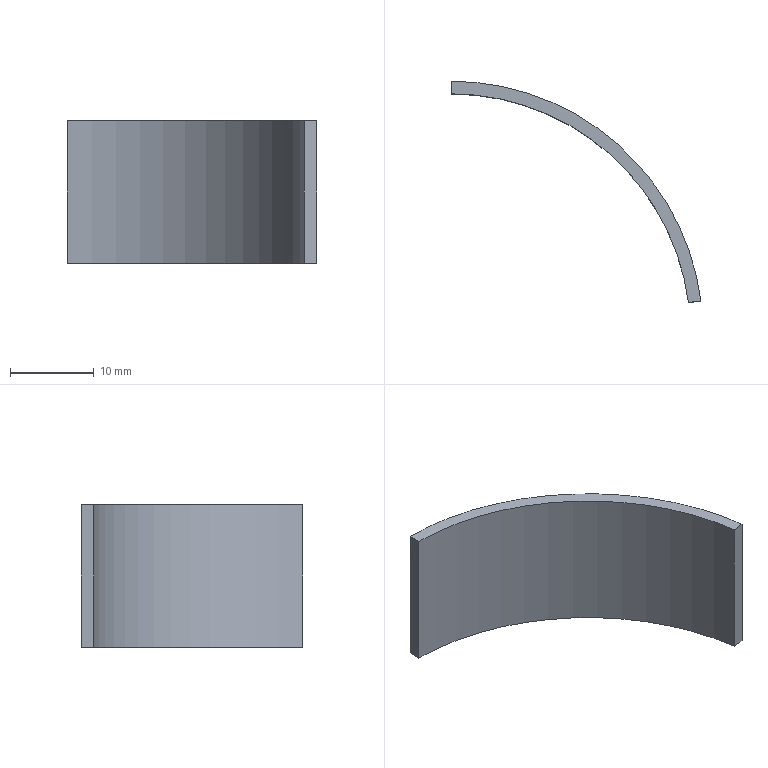Part | STEP file | FHD-021-012-B side door A-B | 1 solid | 6 faces | box 29.753 x 26.353 x 17 mm | volume 1076 mm3 | plane 4 | cylinder 2 | commonest cylinder face diameters 57 x1 60 x1
STEP:
#1=CARTESIAN_POINT('',(0.,0.,0.));
#2=DIRECTION('',(0.,0.,1.));
#3=DIRECTION('',(1.,0.,0.));
#4=AXIS2_PLACEMENT_3D('',#1,#2,#3);
#5=CARTESIAN_POINT('',(1834.327,1290.963,17.));
#6=VERTEX_POINT('',#5);
#7=CARTESIAN_POINT('',(1864.08,1264.802,17.));
#8=VERTEX_POINT('',#7);
#9=CARTESIAN_POINT('',(1834.327,1260.963,17.));
#10=DIRECTION('',(0.,0.,-1.));
#11=DIRECTION('',(-1.,0.,0.));
#12=AXIS2_PLACEMENT_3D('',#9,#10,#11);
#13=CIRCLE('',#12,30.);
#14=CARTESIAN_POINT('',(1834.327,1260.963,17.));
#15=DIRECTION('',(0.,0.,-1.));
#16=DIRECTION('',(-1.,0.,0.));
#17=AXIS2_PLACEMENT_3D('',#14,#15,#16);
#18=CYLINDRICAL_SURFACE('',#17,30.);
#19=CARTESIAN_POINT('',(0.,0.));
#20=DIRECTION('',(1.,0.));
#21=VECTOR('',#20,1.);
#22=LINE('',#19,#21);
#23=(GEOMETRIC_REPRESENTATION_CONTEXT(2)PARAMETRIC_REPRESENTATION_CONTEXT()REPRESENTATION_CONTEXT('',''));
#24=DEFINITIONAL_REPRESENTATION('',(#22),#23);
#25=PCURVE('',#18,#24);
#26=CARTESIAN_POINT('',(1834.327,1260.963,17.));
#27=DIRECTION('',(0.,0.,1.));
#28=DIRECTION('',(1.,0.,0.));
#29=AXIS2_PLACEMENT_3D('',#26,#27,#28);
#30=PLANE('',#29);
#31=CARTESIAN_POINT('',(-30.,0.));
#32=CARTESIAN_POINT('',(-30.,51.962));
#33=CARTESIAN_POINT('',(15.,25.981));
#34=CARTESIAN_POINT('',(60.,0.));
#35=CARTESIAN_POINT('',(15.,-25.981));
#36=CARTESIAN_POINT('',(-30.,-51.962));
#37=CARTESIAN_POINT('',(-30.,0.));
#38=(BOUNDED_CURVE()B_SPLINE_CURVE(2,(#31,#32,#33,#34,#35,#36,#37),.UNSPECIFIED.,.T.,.F.)B_SPLINE_CURVE_WITH_KNOTS((1,2,2,2,2,1),(-2.094,0.,2.094,4.189,6.283,8.378),.UNSPECIFIED.)CURVE()GEOMETRIC_REPRESENTATION_ITEM()RATIONAL_B_SPLINE_CURVE((1.,0.5,1.,0.5,1.,0.5,1.))REPRESENTATION_ITEM(''));
#39=(GEOMETRIC_REPRESENTATION_CONTEXT(2)PARAMETRIC_REPRESENTATION_CONTEXT()REPRESENTATION_CONTEXT('',''));
#40=DEFINITIONAL_REPRESENTATION('',(#38),#39);
#41=PCURVE('',#30,#40);
#42=SURFACE_CURVE('',#13,(#25,#41),.PCURVE_S1.);
#43=EDGE_CURVE('',#6,#8,#42,.T.);
#44=ORIENTED_EDGE('',*,*,#43,.T.);
#45=CARTESIAN_POINT('',(1864.08,1264.802,0.));
#46=VERTEX_POINT('',#45);
#47=CARTESIAN_POINT('',(1864.08,1264.802,17.));
#48=DIRECTION('',(0.,0.,-1.));
#49=VECTOR('',#48,1.);
#50=LINE('',#47,#49);
#51=CARTESIAN_POINT('',(3.013,0.));
#52=DIRECTION('',(0.,1.));
#53=VECTOR('',#52,1.);
#54=LINE('',#51,#53);
#55=(GEOMETRIC_REPRESENTATION_CONTEXT(2)PARAMETRIC_REPRESENTATION_CONTEXT()REPRESENTATION_CONTEXT('',''));
#56=DEFINITIONAL_REPRESENTATION('',(#54),#55);
#57=PCURVE('',#18,#56);
#58=CARTESIAN_POINT('',(1864.08,1264.802,17.));
#59=DIRECTION('',(0.128,-0.9918,0.));
#60=DIRECTION('',(0.9918,0.128,0.));
#61=AXIS2_PLACEMENT_3D('',#58,#59,#60);
#62=PLANE('',#61);
#63=CARTESIAN_POINT('',(0.,0.));
#64=DIRECTION('',(0.,-1.));
#65=VECTOR('',#64,1.);
#66=LINE('',#63,#65);
#67=(GEOMETRIC_REPRESENTATION_CONTEXT(2)PARAMETRIC_REPRESENTATION_CONTEXT()REPRESENTATION_CONTEXT('',''));
#68=DEFINITIONAL_REPRESENTATION('',(#66),#67);
#69=PCURVE('',#62,#68);
#70=SURFACE_CURVE('',#50,(#57,#69),.PCURVE_S1.);
#71=EDGE_CURVE('',#8,#46,#70,.T.);
#72=ORIENTED_EDGE('',*,*,#71,.T.);
#73=CARTESIAN_POINT('',(1834.327,1290.963,0.));
#74=VERTEX_POINT('',#73);
#75=CARTESIAN_POINT('',(1834.327,1260.963,0.));
#76=DIRECTION('',(0.,0.,1.));
#77=DIRECTION('',(-1.,0.,0.));
#78=AXIS2_PLACEMENT_3D('',#75,#76,#77);
#79=CIRCLE('',#78,30.);
#80=CARTESIAN_POINT('',(6.283,17.));
#81=DIRECTION('',(-1.,0.));
#82=VECTOR('',#81,1.);
#83=LINE('',#80,#82);
#84=(GEOMETRIC_REPRESENTATION_CONTEXT(2)PARAMETRIC_REPRESENTATION_CONTEXT()REPRESENTATION_CONTEXT('',''));
#85=DEFINITIONAL_REPRESENTATION('',(#83),#84);
#86=PCURVE('',#18,#85);
#87=CARTESIAN_POINT('',(1834.327,1260.963,0.));
#88=DIRECTION('',(0.,0.,1.));
#89=DIRECTION('',(1.,0.,0.));
#90=AXIS2_PLACEMENT_3D('',#87,#88,#89);
#91=PLANE('',#90);
#92=CARTESIAN_POINT('',(0.,0.));
#93=DIRECTION('',(-1.,0.));
#94=AXIS2_PLACEMENT_2D('',#92,#93);
#95=CIRCLE('',#94,30.);
#96=(GEOMETRIC_REPRESENTATION_CONTEXT(2)PARAMETRIC_REPRESENTATION_CONTEXT()REPRESENTATION_CONTEXT('',''));
#97=DEFINITIONAL_REPRESENTATION('',(#95),#96);
#98=PCURVE('',#91,#97);
#99=SURFACE_CURVE('',#79,(#86,#98),.PCURVE_S1.);
#100=EDGE_CURVE('',#46,#74,#99,.T.);
#101=ORIENTED_EDGE('',*,*,#100,.T.);
#102=CARTESIAN_POINT('',(1834.327,1290.963,17.));
#103=DIRECTION('',(0.,0.,1.));
#104=VECTOR('',#103,1.);
#105=LINE('',#102,#104);
#106=CARTESIAN_POINT('',(1.571,0.));
#107=DIRECTION('',(0.,-1.));
#108=VECTOR('',#107,1.);
#109=LINE('',#106,#108);
#110=(GEOMETRIC_REPRESENTATION_CONTEXT(2)PARAMETRIC_REPRESENTATION_CONTEXT()REPRESENTATION_CONTEXT('',''));
#111=DEFINITIONAL_REPRESENTATION('',(#109),#110);
#112=PCURVE('',#18,#111);
#113=CARTESIAN_POINT('',(1834.327,1289.463,17.));
#114=DIRECTION('',(-1.,0.,0.));
#115=DIRECTION('',(0.,0.,1.));
#116=AXIS2_PLACEMENT_3D('',#113,#114,#115);
#117=PLANE('',#116);
#118=CARTESIAN_POINT('',(0.,1.5));
#119=DIRECTION('',(1.,0.));
#120=VECTOR('',#119,1.);
#121=LINE('',#118,#120);
#122=(GEOMETRIC_REPRESENTATION_CONTEXT(2)PARAMETRIC_REPRESENTATION_CONTEXT()REPRESENTATION_CONTEXT('',''));
#123=DEFINITIONAL_REPRESENTATION('',(#121),#122);
#124=PCURVE('',#117,#123);
#125=SURFACE_CURVE('',#105,(#112,#124),.PCURVE_S1.);
#126=EDGE_CURVE('',#74,#6,#125,.T.);
#127=ORIENTED_EDGE('',*,*,#126,.T.);
#128=EDGE_LOOP('',(#44,#72,#101,#127));
#129=FACE_BOUND('',#128,.T.);
#130=ADVANCED_FACE('',(#129),#18,.T.);
#131=CARTESIAN_POINT('',(1862.593,1264.61,17.));
#132=VERTEX_POINT('',#131);
#133=CARTESIAN_POINT('',(1864.08,1264.802,17.));
#134=DIRECTION('',(-0.9918,-0.128,0.));
#135=VECTOR('',#134,1.);
#136=LINE('',#133,#135);
#137=CARTESIAN_POINT('',(0.,0.));
#138=DIRECTION('',(-1.,0.));
#139=VECTOR('',#138,1.);
#140=LINE('',#137,#139);
#141=(GEOMETRIC_REPRESENTATION_CONTEXT(2)PARAMETRIC_REPRESENTATION_CONTEXT()REPRESENTATION_CONTEXT('',''));
#142=DEFINITIONAL_REPRESENTATION('',(#140),#141);
#143=PCURVE('',#62,#142);
#144=CARTESIAN_POINT('',(29.753,3.839));
#145=DIRECTION('',(-0.9918,-0.128));
#146=VECTOR('',#145,1.);
#147=LINE('',#144,#146);
#148=(GEOMETRIC_REPRESENTATION_CONTEXT(2)PARAMETRIC_REPRESENTATION_CONTEXT()REPRESENTATION_CONTEXT('',''));
#149=DEFINITIONAL_REPRESENTATION('',(#147),#148);
#150=PCURVE('',#30,#149);
#151=SURFACE_CURVE('',#136,(#143,#150),.PCURVE_S1.);
#152=EDGE_CURVE('',#8,#132,#151,.T.);
#153=ORIENTED_EDGE('',*,*,#152,.T.);
#154=CARTESIAN_POINT('',(1862.593,1264.61,0.));
#155=VERTEX_POINT('',#154);
#156=CARTESIAN_POINT('',(1862.593,1264.61,17.));
#157=DIRECTION('',(0.,0.,-1.));
#158=VECTOR('',#157,1.);
#159=LINE('',#156,#158);
#160=CARTESIAN_POINT('',(-1.5,0.));
#161=DIRECTION('',(0.,-1.));
#162=VECTOR('',#161,1.);
#163=LINE('',#160,#162);
#164=(GEOMETRIC_REPRESENTATION_CONTEXT(2)PARAMETRIC_REPRESENTATION_CONTEXT()REPRESENTATION_CONTEXT('',''));
#165=DEFINITIONAL_REPRESENTATION('',(#163),#164);
#166=PCURVE('',#62,#165);
#167=CARTESIAN_POINT('',(1834.327,1260.963,17.));
#168=DIRECTION('',(0.,0.,-1.));
#169=DIRECTION('',(-1.,0.,0.));
#170=AXIS2_PLACEMENT_3D('',#167,#168,#169);
#171=CYLINDRICAL_SURFACE('',#170,28.5);
#172=CARTESIAN_POINT('',(3.013,0.));
#173=DIRECTION('',(0.,1.));
#174=VECTOR('',#173,1.);
#175=LINE('',#172,#174);
#176=(GEOMETRIC_REPRESENTATION_CONTEXT(2)PARAMETRIC_REPRESENTATION_CONTEXT()REPRESENTATION_CONTEXT('',''));
#177=DEFINITIONAL_REPRESENTATION('',(#175),#176);
#178=PCURVE('',#171,#177);
#179=SURFACE_CURVE('',#159,(#166,#178),.PCURVE_S1.);
#180=EDGE_CURVE('',#132,#155,#179,.T.);
#181=ORIENTED_EDGE('',*,*,#180,.T.);
#182=CARTESIAN_POINT('',(1864.08,1264.802,0.));
#183=DIRECTION('',(0.9918,0.128,0.));
#184=VECTOR('',#183,1.);
#185=LINE('',#182,#184);
#186=CARTESIAN_POINT('',(0.,-17.));
#187=DIRECTION('',(1.,0.));
#188=VECTOR('',#187,1.);
#189=LINE('',#186,#188);
#190=(GEOMETRIC_REPRESENTATION_CONTEXT(2)PARAMETRIC_REPRESENTATION_CONTEXT()REPRESENTATION_CONTEXT('',''));
#191=DEFINITIONAL_REPRESENTATION('',(#189),#190);
#192=PCURVE('',#62,#191);
#193=CARTESIAN_POINT('',(29.753,3.839));
#194=DIRECTION('',(0.9918,0.128));
#195=VECTOR('',#194,1.);
#196=LINE('',#193,#195);
#197=(GEOMETRIC_REPRESENTATION_CONTEXT(2)PARAMETRIC_REPRESENTATION_CONTEXT()REPRESENTATION_CONTEXT('',''));
#198=DEFINITIONAL_REPRESENTATION('',(#196),#197);
#199=PCURVE('',#91,#198);
#200=SURFACE_CURVE('',#185,(#192,#199),.PCURVE_S1.);
#201=EDGE_CURVE('',#155,#46,#200,.T.);
#202=ORIENTED_EDGE('',*,*,#201,.T.);
#203=ORIENTED_EDGE('',*,*,#71,.F.);
#204=EDGE_LOOP('',(#153,#181,#202,#203));
#205=FACE_BOUND('',#204,.T.);
#206=ADVANCED_FACE('',(#205),#62,.T.);
#207=CARTESIAN_POINT('',(1834.327,1289.463,17.));
#208=VERTEX_POINT('',#207);
#209=CARTESIAN_POINT('',(1834.327,1260.963,17.));
#210=DIRECTION('',(0.,0.,-1.));
#211=DIRECTION('',(-1.,0.,0.));
#212=AXIS2_PLACEMENT_3D('',#209,#210,#211);
#213=CIRCLE('',#212,28.5);
#214=CARTESIAN_POINT('',(-28.5,0.));
#215=CARTESIAN_POINT('',(-28.5,49.363));
#216=CARTESIAN_POINT('',(14.25,24.682));
#217=CARTESIAN_POINT('',(57.,0.));
#218=CARTESIAN_POINT('',(14.25,-24.682));
#219=CARTESIAN_POINT('',(-28.5,-49.363));
#220=CARTESIAN_POINT('',(-28.5,0.));
#221=(BOUNDED_CURVE()B_SPLINE_CURVE(2,(#214,#215,#216,#217,#218,#219,#220),.UNSPECIFIED.,.T.,.F.)B_SPLINE_CURVE_WITH_KNOTS((1,2,2,2,2,1),(-2.094,0.,2.094,4.189,6.283,8.378),.UNSPECIFIED.)CURVE()GEOMETRIC_REPRESENTATION_ITEM()RATIONAL_B_SPLINE_CURVE((1.,0.5,1.,0.5,1.,0.5,1.))REPRESENTATION_ITEM(''));
#222=(GEOMETRIC_REPRESENTATION_CONTEXT(2)PARAMETRIC_REPRESENTATION_CONTEXT()REPRESENTATION_CONTEXT('',''));
#223=DEFINITIONAL_REPRESENTATION('',(#221),#222);
#224=PCURVE('',#30,#223);
#225=CARTESIAN_POINT('',(0.,0.));
#226=DIRECTION('',(1.,0.));
#227=VECTOR('',#226,1.);
#228=LINE('',#225,#227);
#229=(GEOMETRIC_REPRESENTATION_CONTEXT(2)PARAMETRIC_REPRESENTATION_CONTEXT()REPRESENTATION_CONTEXT('',''));
#230=DEFINITIONAL_REPRESENTATION('',(#228),#229);
#231=PCURVE('',#171,#230);
#232=SURFACE_CURVE('',#213,(#224,#231),.PCURVE_S1.);
#233=EDGE_CURVE('',#208,#132,#232,.T.);
#234=ORIENTED_EDGE('',*,*,#233,.T.);
#235=ORIENTED_EDGE('',*,*,#152,.F.);
#236=ORIENTED_EDGE('',*,*,#43,.F.);
#237=CARTESIAN_POINT('',(1834.327,1260.963,17.));
#238=DIRECTION('',(0.,-1.,0.));
#239=VECTOR('',#238,1.);
#240=LINE('',#237,#239);
#241=CARTESIAN_POINT('',(0.,0.));
#242=DIRECTION('',(0.,-1.));
#243=VECTOR('',#242,1.);
#244=LINE('',#241,#243);
#245=(GEOMETRIC_REPRESENTATION_CONTEXT(2)PARAMETRIC_REPRESENTATION_CONTEXT()REPRESENTATION_CONTEXT('',''));
#246=DEFINITIONAL_REPRESENTATION('',(#244),#245);
#247=PCURVE('',#30,#246);
#248=CARTESIAN_POINT('',(0.,-28.5));
#249=DIRECTION('',(0.,-1.));
#250=VECTOR('',#249,1.);
#251=LINE('',#248,#250);
#252=(GEOMETRIC_REPRESENTATION_CONTEXT(2)PARAMETRIC_REPRESENTATION_CONTEXT()REPRESENTATION_CONTEXT('',''));
#253=DEFINITIONAL_REPRESENTATION('',(#251),#252);
#254=PCURVE('',#117,#253);
#255=SURFACE_CURVE('',#240,(#247,#254),.PCURVE_S1.);
#256=EDGE_CURVE('',#6,#208,#255,.T.);
#257=ORIENTED_EDGE('',*,*,#256,.T.);
#258=EDGE_LOOP('',(#234,#235,#236,#257));
#259=FACE_BOUND('',#258,.T.);
#260=ADVANCED_FACE('',(#259),#30,.T.);
#261=ORIENTED_EDGE('',*,*,#256,.F.);
#262=ORIENTED_EDGE('',*,*,#126,.F.);
#263=CARTESIAN_POINT('',(1834.327,1289.463,0.));
#264=VERTEX_POINT('',#263);
#265=CARTESIAN_POINT('',(1834.327,1289.463,0.));
#266=DIRECTION('',(0.,-1.,0.));
#267=VECTOR('',#266,1.);
#268=LINE('',#265,#267);
#269=CARTESIAN_POINT('',(-17.,0.));
#270=DIRECTION('',(0.,-1.));
#271=VECTOR('',#270,1.);
#272=LINE('',#269,#271);
#273=(GEOMETRIC_REPRESENTATION_CONTEXT(2)PARAMETRIC_REPRESENTATION_CONTEXT()REPRESENTATION_CONTEXT('',''));
#274=DEFINITIONAL_REPRESENTATION('',(#272),#273);
#275=PCURVE('',#117,#274);
#276=CARTESIAN_POINT('',(0.,28.5));
#277=DIRECTION('',(0.,-1.));
#278=VECTOR('',#277,1.);
#279=LINE('',#276,#278);
#280=(GEOMETRIC_REPRESENTATION_CONTEXT(2)PARAMETRIC_REPRESENTATION_CONTEXT()REPRESENTATION_CONTEXT('',''));
#281=DEFINITIONAL_REPRESENTATION('',(#279),#280);
#282=PCURVE('',#91,#281);
#283=SURFACE_CURVE('',#268,(#275,#282),.PCURVE_S1.);
#284=EDGE_CURVE('',#74,#264,#283,.T.);
#285=ORIENTED_EDGE('',*,*,#284,.T.);
#286=CARTESIAN_POINT('',(1834.327,1289.463,17.));
#287=DIRECTION('',(0.,0.,1.));
#288=VECTOR('',#287,1.);
#289=LINE('',#286,#288);
#290=CARTESIAN_POINT('',(0.,0.));
#291=DIRECTION('',(1.,0.));
#292=VECTOR('',#291,1.);
#293=LINE('',#290,#292);
#294=(GEOMETRIC_REPRESENTATION_CONTEXT(2)PARAMETRIC_REPRESENTATION_CONTEXT()REPRESENTATION_CONTEXT('',''));
#295=DEFINITIONAL_REPRESENTATION('',(#293),#294);
#296=PCURVE('',#117,#295);
#297=CARTESIAN_POINT('',(1.571,0.));
#298=DIRECTION('',(0.,-1.));
#299=VECTOR('',#298,1.);
#300=LINE('',#297,#299);
#301=(GEOMETRIC_REPRESENTATION_CONTEXT(2)PARAMETRIC_REPRESENTATION_CONTEXT()REPRESENTATION_CONTEXT('',''));
#302=DEFINITIONAL_REPRESENTATION('',(#300),#301);
#303=PCURVE('',#171,#302);
#304=SURFACE_CURVE('',#289,(#296,#303),.PCURVE_S1.);
#305=EDGE_CURVE('',#264,#208,#304,.T.);
#306=ORIENTED_EDGE('',*,*,#305,.T.);
#307=EDGE_LOOP('',(#261,#262,#285,#306));
#308=FACE_BOUND('',#307,.T.);
#309=ADVANCED_FACE('',(#308),#117,.T.);
#310=ORIENTED_EDGE('',*,*,#201,.F.);
#311=CARTESIAN_POINT('',(1834.327,1260.963,0.));
#312=DIRECTION('',(0.,0.,-1.));
#313=DIRECTION('',(-1.,0.,0.));
#314=AXIS2_PLACEMENT_3D('',#311,#312,#313);
#315=CIRCLE('',#314,28.5);
#316=CARTESIAN_POINT('',(-28.5,0.));
#317=CARTESIAN_POINT('',(-28.5,49.363));
#318=CARTESIAN_POINT('',(14.25,24.682));
#319=CARTESIAN_POINT('',(57.,0.));
#320=CARTESIAN_POINT('',(14.25,-24.682));
#321=CARTESIAN_POINT('',(-28.5,-49.363));
#322=CARTESIAN_POINT('',(-28.5,0.));
#323=(BOUNDED_CURVE()B_SPLINE_CURVE(2,(#316,#317,#318,#319,#320,#321,#322),.UNSPECIFIED.,.T.,.F.)B_SPLINE_CURVE_WITH_KNOTS((1,2,2,2,2,1),(-2.094,0.,2.094,4.189,6.283,8.378),.UNSPECIFIED.)CURVE()GEOMETRIC_REPRESENTATION_ITEM()RATIONAL_B_SPLINE_CURVE((1.,0.5,1.,0.5,1.,0.5,1.))REPRESENTATION_ITEM(''));
#324=(GEOMETRIC_REPRESENTATION_CONTEXT(2)PARAMETRIC_REPRESENTATION_CONTEXT()REPRESENTATION_CONTEXT('',''));
#325=DEFINITIONAL_REPRESENTATION('',(#323),#324);
#326=PCURVE('',#91,#325);
#327=CARTESIAN_POINT('',(0.,17.));
#328=DIRECTION('',(1.,0.));
#329=VECTOR('',#328,1.);
#330=LINE('',#327,#329);
#331=(GEOMETRIC_REPRESENTATION_CONTEXT(2)PARAMETRIC_REPRESENTATION_CONTEXT()REPRESENTATION_CONTEXT('',''));
#332=DEFINITIONAL_REPRESENTATION('',(#330),#331);
#333=PCURVE('',#171,#332);
#334=SURFACE_CURVE('',#315,(#326,#333),.PCURVE_S1.);
#335=EDGE_CURVE('',#264,#155,#334,.T.);
#336=ORIENTED_EDGE('',*,*,#335,.F.);
#337=ORIENTED_EDGE('',*,*,#284,.F.);
#338=ORIENTED_EDGE('',*,*,#100,.F.);
#339=EDGE_LOOP('',(#310,#336,#337,#338));
#340=FACE_BOUND('',#339,.T.);
#341=ADVANCED_FACE('',(#340),#91,.F.);
#342=ORIENTED_EDGE('',*,*,#335,.F.);
#343=ORIENTED_EDGE('',*,*,#305,.T.);
#344=ORIENTED_EDGE('',*,*,#233,.T.);
#345=ORIENTED_EDGE('',*,*,#180,.T.);
#346=EDGE_LOOP('',(#342,#343,#344,#345));
#347=FACE_BOUND('',#346,.F.);
#348=ADVANCED_FACE('',(#347),#171,.F.);
#349=CLOSED_SHELL('',(#130,#206,#260,#309,#341,#348));
#350=MANIFOLD_SOLID_BREP('',#349);
#351=(LENGTH_UNIT()NAMED_UNIT(*)SI_UNIT(.MILLI.,.METRE.));
#352=UNCERTAINTY_MEASURE_WITH_UNIT(LENGTH_MEASURE(0.0000001),#351,'','');
#353=(NAMED_UNIT(*)PLANE_ANGLE_UNIT()SI_UNIT($,.RADIAN.));
#354=(NAMED_UNIT(*)SI_UNIT($,.STERADIAN.)SOLID_ANGLE_UNIT());
#355=(GEOMETRIC_REPRESENTATION_CONTEXT(3)GLOBAL_UNCERTAINTY_ASSIGNED_CONTEXT((#352))GLOBAL_UNIT_ASSIGNED_CONTEXT((#351,#353,#354))REPRESENTATION_CONTEXT('',''));
#356=ADVANCED_BREP_SHAPE_REPRESENTATION('',(#4,#350),#355);